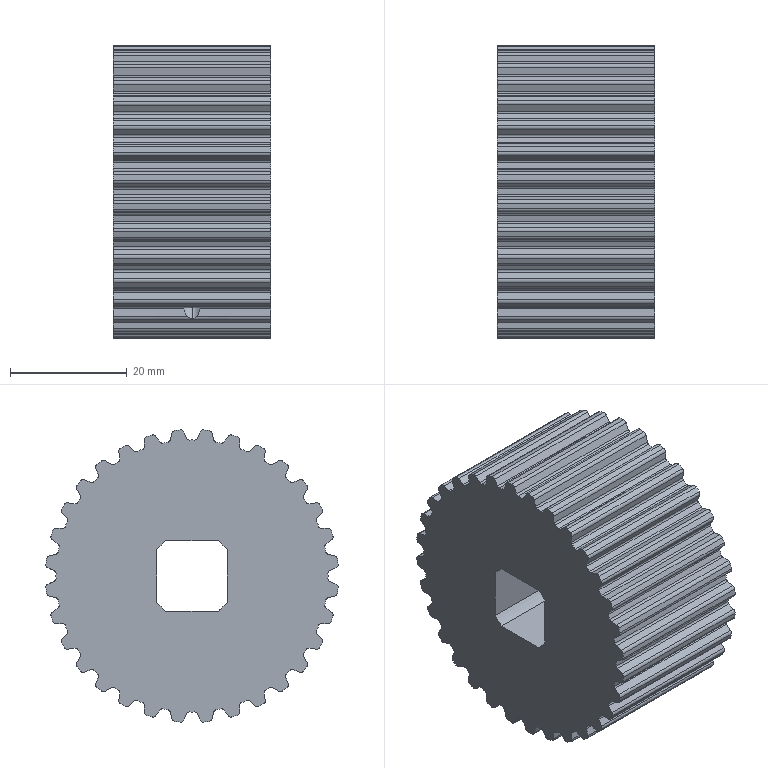Part | STEP file | TTPP32T5250-A-P11_b transition pulley | 1 solid | 285 faces | box 27 x 49.946 x 49.946 mm | volume 37850 mm3 | cylinder 208 | plane 75 | torus 2 | commonest cylinder face diameters 0.8 x68 1.2 x64 46.5 x34 50.1 x32 3.242 x4 15 x4